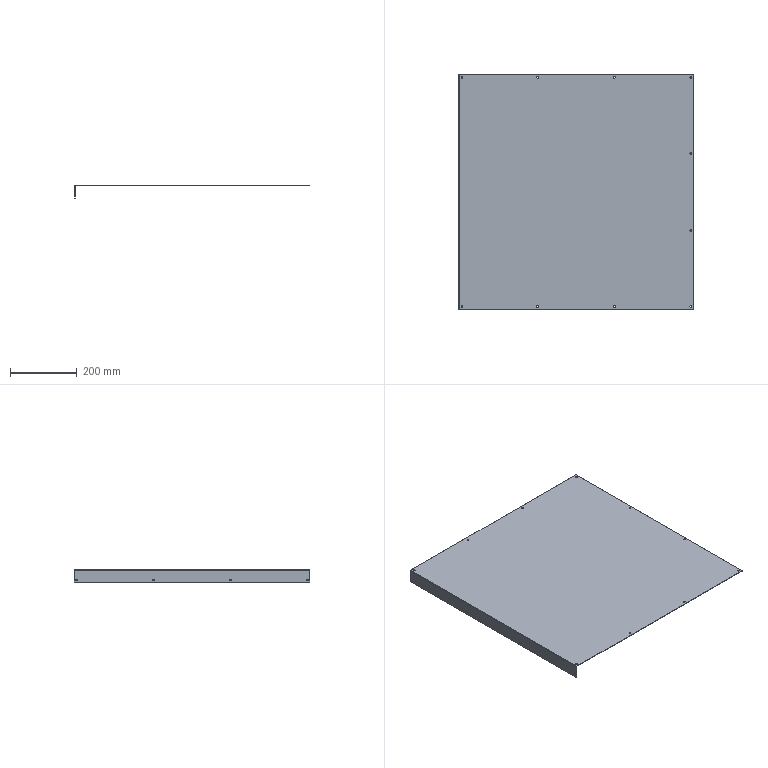Part | SolidWorks | features HoleWzd 2, EdgeFlange 1, Fillet 1, FlatPattern 1, SMBaseFlange 1, SheetMetal 1 | 1 solid | 46 faces | box 703 x 704 x 40 mm | volume 781813 mm3 | cylinder 34 | plane 12 | commonest cylinder face diameters 5 x29 4 x4 2 x1
STEP:
#1=CARTESIAN_POINT('',(-344.,-343.,-1.5));
#2=VERTEX_POINT('',#1);
#3=CARTESIAN_POINT('',(-339.,-343.,-1.5));
#4=VERTEX_POINT('',#3);
#5=CARTESIAN_POINT('',(-341.5,-343.,-1.5));
#6=DIRECTION('',(0.,0.,1.));
#7=DIRECTION('',(1.,0.,0.));
#8=AXIS2_PLACEMENT_3D('',#5,#6,#7);
#9=CIRCLE('',#8,2.5);
#10=EDGE_CURVE('',#2,#4,#9,.T.);
#11=ORIENTED_EDGE('',*,*,#10,.F.);
#12=CARTESIAN_POINT('',(-344.,-343.,0.));
#13=VERTEX_POINT('',#12);
#14=CARTESIAN_POINT('',(-344.,-343.,0.));
#15=DIRECTION('',(0.,0.,1.));
#16=VECTOR('',#15,1000.);
#17=LINE('',#14,#16);
#18=EDGE_CURVE('',#2,#13,#17,.T.);
#19=ORIENTED_EDGE('',*,*,#18,.T.);
#20=CARTESIAN_POINT('',(-339.,-343.,0.));
#21=VERTEX_POINT('',#20);
#22=CARTESIAN_POINT('',(-341.5,-343.,0.));
#23=DIRECTION('',(0.,0.,1.));
#24=DIRECTION('',(1.,0.,0.));
#25=AXIS2_PLACEMENT_3D('',#22,#23,#24);
#26=CIRCLE('',#25,2.5);
#27=EDGE_CURVE('',#13,#21,#26,.T.);
#28=ORIENTED_EDGE('',*,*,#27,.T.);
#29=CARTESIAN_POINT('',(-339.,-343.,0.));
#30=DIRECTION('',(0.,0.,1.));
#31=VECTOR('',#30,1000.);
#32=LINE('',#29,#31);
#33=EDGE_CURVE('',#4,#21,#32,.T.);
#34=ORIENTED_EDGE('',*,*,#33,.F.);
#35=EDGE_LOOP('',(#11,#19,#28,#34));
#36=FACE_OUTER_BOUND('',#35,.T.);
#37=CARTESIAN_POINT('',(-341.5,-343.,0.));
#38=DIRECTION('',(0.,0.,1.));
#39=DIRECTION('',(1.,0.,0.));
#40=AXIS2_PLACEMENT_3D('',#37,#38,#39);
#41=CYLINDRICAL_SURFACE('',#40,2.5);
#42=ADVANCED_FACE('',(#36),#41,.F.);
#43=CARTESIAN_POINT('',(-117.5,-343.,-1.5));
#44=VERTEX_POINT('',#43);
#45=CARTESIAN_POINT('',(-112.5,-343.,-1.5));
#46=VERTEX_POINT('',#45);
#47=CARTESIAN_POINT('',(-115.,-343.,-1.5));
#48=DIRECTION('',(0.,0.,1.));
#49=DIRECTION('',(1.,0.,0.));
#50=AXIS2_PLACEMENT_3D('',#47,#48,#49);
#51=CIRCLE('',#50,2.5);
#52=EDGE_CURVE('',#44,#46,#51,.T.);
#53=ORIENTED_EDGE('',*,*,#52,.F.);
#54=CARTESIAN_POINT('',(-117.5,-343.,0.));
#55=VERTEX_POINT('',#54);
#56=CARTESIAN_POINT('',(-117.5,-343.,0.));
#57=DIRECTION('',(0.,0.,1.));
#58=VECTOR('',#57,1000.);
#59=LINE('',#56,#58);
#60=EDGE_CURVE('',#44,#55,#59,.T.);
#61=ORIENTED_EDGE('',*,*,#60,.T.);
#62=CARTESIAN_POINT('',(-112.5,-343.,0.));
#63=VERTEX_POINT('',#62);
#64=CARTESIAN_POINT('',(-115.,-343.,0.));
#65=DIRECTION('',(0.,0.,1.));
#66=DIRECTION('',(1.,0.,0.));
#67=AXIS2_PLACEMENT_3D('',#64,#65,#66);
#68=CIRCLE('',#67,2.5);
#69=EDGE_CURVE('',#55,#63,#68,.T.);
#70=ORIENTED_EDGE('',*,*,#69,.T.);
#71=CARTESIAN_POINT('',(-112.5,-343.,0.));
#72=DIRECTION('',(0.,0.,1.));
#73=VECTOR('',#72,1000.);
#74=LINE('',#71,#73);
#75=EDGE_CURVE('',#46,#63,#74,.T.);
#76=ORIENTED_EDGE('',*,*,#75,.F.);
#77=EDGE_LOOP('',(#53,#61,#70,#76));
#78=FACE_OUTER_BOUND('',#77,.T.);
#79=CARTESIAN_POINT('',(-115.,-343.,0.));
#80=DIRECTION('',(0.,0.,1.));
#81=DIRECTION('',(1.,0.,0.));
#82=AXIS2_PLACEMENT_3D('',#79,#80,#81);
#83=CYLINDRICAL_SURFACE('',#82,2.5);
#84=ADVANCED_FACE('',(#78),#83,.F.);
#85=CARTESIAN_POINT('',(112.5,-343.,-1.5));
#86=VERTEX_POINT('',#85);
#87=CARTESIAN_POINT('',(117.5,-343.,-1.5));
#88=VERTEX_POINT('',#87);
#89=CARTESIAN_POINT('',(115.,-343.,-1.5));
#90=DIRECTION('',(0.,0.,1.));
#91=DIRECTION('',(1.,0.,0.));
#92=AXIS2_PLACEMENT_3D('',#89,#90,#91);
#93=CIRCLE('',#92,2.5);
#94=EDGE_CURVE('',#86,#88,#93,.T.);
#95=ORIENTED_EDGE('',*,*,#94,.F.);
#96=CARTESIAN_POINT('',(112.5,-343.,0.));
#97=VERTEX_POINT('',#96);
#98=CARTESIAN_POINT('',(112.5,-343.,0.));
#99=DIRECTION('',(0.,0.,1.));
#100=VECTOR('',#99,1000.);
#101=LINE('',#98,#100);
#102=EDGE_CURVE('',#86,#97,#101,.T.);
#103=ORIENTED_EDGE('',*,*,#102,.T.);
#104=CARTESIAN_POINT('',(117.5,-343.,0.));
#105=VERTEX_POINT('',#104);
#106=CARTESIAN_POINT('',(115.,-343.,0.));
#107=DIRECTION('',(0.,0.,1.));
#108=DIRECTION('',(1.,0.,0.));
#109=AXIS2_PLACEMENT_3D('',#106,#107,#108);
#110=CIRCLE('',#109,2.5);
#111=EDGE_CURVE('',#97,#105,#110,.T.);
#112=ORIENTED_EDGE('',*,*,#111,.T.);
#113=CARTESIAN_POINT('',(117.5,-343.,0.));
#114=DIRECTION('',(0.,0.,1.));
#115=VECTOR('',#114,1000.);
#116=LINE('',#113,#115);
#117=EDGE_CURVE('',#88,#105,#116,.T.);
#118=ORIENTED_EDGE('',*,*,#117,.F.);
#119=EDGE_LOOP('',(#95,#103,#112,#118));
#120=FACE_OUTER_BOUND('',#119,.T.);
#121=CARTESIAN_POINT('',(115.,-343.,0.));
#122=DIRECTION('',(0.,0.,1.));
#123=DIRECTION('',(1.,0.,0.));
#124=AXIS2_PLACEMENT_3D('',#121,#122,#123);
#125=CYLINDRICAL_SURFACE('',#124,2.5);
#126=ADVANCED_FACE('',(#120),#125,.F.);
#127=CARTESIAN_POINT('',(341.,-343.,-1.5));
#128=VERTEX_POINT('',#127);
#129=CARTESIAN_POINT('',(346.,-343.,-1.5));
#130=VERTEX_POINT('',#129);
#131=CARTESIAN_POINT('',(343.5,-343.,-1.5));
#132=DIRECTION('',(0.,0.,1.));
#133=DIRECTION('',(1.,0.,0.));
#134=AXIS2_PLACEMENT_3D('',#131,#132,#133);
#135=CIRCLE('',#134,2.5);
#136=EDGE_CURVE('',#128,#130,#135,.T.);
#137=ORIENTED_EDGE('',*,*,#136,.F.);
#138=CARTESIAN_POINT('',(341.,-343.,0.));
#139=VERTEX_POINT('',#138);
#140=CARTESIAN_POINT('',(341.,-343.,0.));
#141=DIRECTION('',(0.,0.,1.));
#142=VECTOR('',#141,1000.);
#143=LINE('',#140,#142);
#144=EDGE_CURVE('',#128,#139,#143,.T.);
#145=ORIENTED_EDGE('',*,*,#144,.T.);
#146=CARTESIAN_POINT('',(346.,-343.,0.));
#147=VERTEX_POINT('',#146);
#148=CARTESIAN_POINT('',(343.5,-343.,0.));
#149=DIRECTION('',(0.,0.,1.));
#150=DIRECTION('',(1.,0.,0.));
#151=AXIS2_PLACEMENT_3D('',#148,#149,#150);
#152=CIRCLE('',#151,2.5);
#153=EDGE_CURVE('',#139,#147,#152,.T.);
#154=ORIENTED_EDGE('',*,*,#153,.T.);
#155=CARTESIAN_POINT('',(346.,-343.,0.));
#156=DIRECTION('',(0.,0.,1.));
#157=VECTOR('',#156,1000.);
#158=LINE('',#155,#157);
#159=EDGE_CURVE('',#130,#147,#158,.T.);
#160=ORIENTED_EDGE('',*,*,#159,.F.);
#161=EDGE_LOOP('',(#137,#145,#154,#160));
#162=FACE_OUTER_BOUND('',#161,.T.);
#163=CARTESIAN_POINT('',(343.5,-343.,0.));
#164=DIRECTION('',(0.,0.,1.));
#165=DIRECTION('',(1.,0.,0.));
#166=AXIS2_PLACEMENT_3D('',#163,#164,#165);
#167=CYLINDRICAL_SURFACE('',#166,2.5);
#168=ADVANCED_FACE('',(#162),#167,.F.);
#169=CARTESIAN_POINT('',(341.,-115.,-1.5));
#170=VERTEX_POINT('',#169);
#171=CARTESIAN_POINT('',(346.,-115.,-1.5));
#172=VERTEX_POINT('',#171);
#173=CARTESIAN_POINT('',(343.5,-115.,-1.5));
#174=DIRECTION('',(0.,0.,1.));
#175=DIRECTION('',(1.,0.,0.));
#176=AXIS2_PLACEMENT_3D('',#173,#174,#175);
#177=CIRCLE('',#176,2.5);
#178=EDGE_CURVE('',#170,#172,#177,.T.);
#179=ORIENTED_EDGE('',*,*,#178,.F.);
#180=CARTESIAN_POINT('',(341.,-115.,0.));
#181=VERTEX_POINT('',#180);
#182=CARTESIAN_POINT('',(341.,-115.,0.));
#183=DIRECTION('',(0.,0.,1.));
#184=VECTOR('',#183,1000.);
#185=LINE('',#182,#184);
#186=EDGE_CURVE('',#170,#181,#185,.T.);
#187=ORIENTED_EDGE('',*,*,#186,.T.);
#188=CARTESIAN_POINT('',(346.,-115.,0.));
#189=VERTEX_POINT('',#188);
#190=CARTESIAN_POINT('',(343.5,-115.,0.));
#191=DIRECTION('',(0.,0.,1.));
#192=DIRECTION('',(1.,0.,0.));
#193=AXIS2_PLACEMENT_3D('',#190,#191,#192);
#194=CIRCLE('',#193,2.5);
#195=EDGE_CURVE('',#181,#189,#194,.T.);
#196=ORIENTED_EDGE('',*,*,#195,.T.);
#197=CARTESIAN_POINT('',(346.,-115.,0.));
#198=DIRECTION('',(0.,0.,1.));
#199=VECTOR('',#198,1000.);
#200=LINE('',#197,#199);
#201=EDGE_CURVE('',#172,#189,#200,.T.);
#202=ORIENTED_EDGE('',*,*,#201,.F.);
#203=EDGE_LOOP('',(#179,#187,#196,#202));
#204=FACE_OUTER_BOUND('',#203,.T.);
#205=CARTESIAN_POINT('',(343.5,-115.,0.));
#206=DIRECTION('',(0.,0.,1.));
#207=DIRECTION('',(1.,0.,0.));
#208=AXIS2_PLACEMENT_3D('',#205,#206,#207);
#209=CYLINDRICAL_SURFACE('',#208,2.5);
#210=ADVANCED_FACE('',(#204),#209,.F.);
#211=CARTESIAN_POINT('',(341.,115.,-1.5));
#212=VERTEX_POINT('',#211);
#213=CARTESIAN_POINT('',(346.,115.,-1.5));
#214=VERTEX_POINT('',#213);
#215=CARTESIAN_POINT('',(343.5,115.,-1.5));
#216=DIRECTION('',(0.,0.,1.));
#217=DIRECTION('',(1.,0.,0.));
#218=AXIS2_PLACEMENT_3D('',#215,#216,#217);
#219=CIRCLE('',#218,2.5);
#220=EDGE_CURVE('',#212,#214,#219,.T.);
#221=ORIENTED_EDGE('',*,*,#220,.F.);
#222=CARTESIAN_POINT('',(341.,115.,0.));
#223=VERTEX_POINT('',#222);
#224=CARTESIAN_POINT('',(341.,115.,0.));
#225=DIRECTION('',(0.,0.,1.));
#226=VECTOR('',#225,1000.);
#227=LINE('',#224,#226);
#228=EDGE_CURVE('',#212,#223,#227,.T.);
#229=ORIENTED_EDGE('',*,*,#228,.T.);
#230=CARTESIAN_POINT('',(346.,115.,0.));
#231=VERTEX_POINT('',#230);
#232=CARTESIAN_POINT('',(343.5,115.,0.));
#233=DIRECTION('',(0.,0.,1.));
#234=DIRECTION('',(1.,0.,0.));
#235=AXIS2_PLACEMENT_3D('',#232,#233,#234);
#236=CIRCLE('',#235,2.5);
#237=EDGE_CURVE('',#223,#231,#236,.T.);
#238=ORIENTED_EDGE('',*,*,#237,.T.);
#239=CARTESIAN_POINT('',(346.,115.,0.));
#240=DIRECTION('',(0.,0.,1.));
#241=VECTOR('',#240,1000.);
#242=LINE('',#239,#241);
#243=EDGE_CURVE('',#214,#231,#242,.T.);
#244=ORIENTED_EDGE('',*,*,#243,.F.);
#245=EDGE_LOOP('',(#221,#229,#238,#244));
#246=FACE_OUTER_BOUND('',#245,.T.);
#247=CARTESIAN_POINT('',(343.5,115.,0.));
#248=DIRECTION('',(0.,0.,1.));
#249=DIRECTION('',(1.,0.,0.));
#250=AXIS2_PLACEMENT_3D('',#247,#248,#249);
#251=CYLINDRICAL_SURFACE('',#250,2.5);
#252=ADVANCED_FACE('',(#246),#251,.F.);
#253=CARTESIAN_POINT('',(341.,343.,-1.5));
#254=VERTEX_POINT('',#253);
#255=CARTESIAN_POINT('',(346.,343.,-1.5));
#256=VERTEX_POINT('',#255);
#257=CARTESIAN_POINT('',(343.5,343.,-1.5));
#258=DIRECTION('',(0.,0.,1.));
#259=DIRECTION('',(1.,0.,0.));
#260=AXIS2_PLACEMENT_3D('',#257,#258,#259);
#261=CIRCLE('',#260,2.5);
#262=EDGE_CURVE('',#254,#256,#261,.T.);
#263=ORIENTED_EDGE('',*,*,#262,.F.);
#264=CARTESIAN_POINT('',(341.,343.,0.));
#265=VERTEX_POINT('',#264);
#266=CARTESIAN_POINT('',(341.,343.,0.));
#267=DIRECTION('',(0.,0.,1.));
#268=VECTOR('',#267,1000.);
#269=LINE('',#266,#268);
#270=EDGE_CURVE('',#254,#265,#269,.T.);
#271=ORIENTED_EDGE('',*,*,#270,.T.);
#272=CARTESIAN_POINT('',(346.,343.,0.));
#273=VERTEX_POINT('',#272);
#274=CARTESIAN_POINT('',(343.5,343.,0.));
#275=DIRECTION('',(0.,0.,1.));
#276=DIRECTION('',(1.,0.,0.));
#277=AXIS2_PLACEMENT_3D('',#274,#275,#276);
#278=CIRCLE('',#277,2.5);
#279=EDGE_CURVE('',#265,#273,#278,.T.);
#280=ORIENTED_EDGE('',*,*,#279,.T.);
#281=CARTESIAN_POINT('',(346.,343.,0.));
#282=DIRECTION('',(0.,0.,1.));
#283=VECTOR('',#282,1000.);
#284=LINE('',#281,#283);
#285=EDGE_CURVE('',#256,#273,#284,.T.);
#286=ORIENTED_EDGE('',*,*,#285,.F.);
#287=EDGE_LOOP('',(#263,#271,#280,#286));
#288=FACE_OUTER_BOUND('',#287,.T.);
#289=CARTESIAN_POINT('',(343.5,343.,0.));
#290=DIRECTION('',(0.,0.,1.));
#291=DIRECTION('',(1.,0.,0.));
#292=AXIS2_PLACEMENT_3D('',#289,#290,#291);
#293=CYLINDRICAL_SURFACE('',#292,2.5);
#294=ADVANCED_FACE('',(#288),#293,.F.);
#295=CARTESIAN_POINT('',(112.5,343.,-1.5));
#296=VERTEX_POINT('',#295);
#297=CARTESIAN_POINT('',(117.5,343.,-1.5));
#298=VERTEX_POINT('',#297);
#299=CARTESIAN_POINT('',(115.,343.,-1.5));
#300=DIRECTION('',(0.,0.,1.));
#301=DIRECTION('',(1.,0.,0.));
#302=AXIS2_PLACEMENT_3D('',#299,#300,#301);
#303=CIRCLE('',#302,2.5);
#304=EDGE_CURVE('',#296,#298,#303,.T.);
#305=ORIENTED_EDGE('',*,*,#304,.F.);
#306=CARTESIAN_POINT('',(112.5,343.,0.));
#307=VERTEX_POINT('',#306);
#308=CARTESIAN_POINT('',(112.5,343.,0.));
#309=DIRECTION('',(0.,0.,1.));
#310=VECTOR('',#309,1000.);
#311=LINE('',#308,#310);
#312=EDGE_CURVE('',#296,#307,#311,.T.);
#313=ORIENTED_EDGE('',*,*,#312,.T.);
#314=CARTESIAN_POINT('',(117.5,343.,0.));
#315=VERTEX_POINT('',#314);
#316=CARTESIAN_POINT('',(115.,343.,0.));
#317=DIRECTION('',(0.,0.,1.));
#318=DIRECTION('',(1.,0.,0.));
#319=AXIS2_PLACEMENT_3D('',#316,#317,#318);
#320=CIRCLE('',#319,2.5);
#321=EDGE_CURVE('',#307,#315,#320,.T.);
#322=ORIENTED_EDGE('',*,*,#321,.T.);
#323=CARTESIAN_POINT('',(117.5,343.,0.));
#324=DIRECTION('',(0.,0.,1.));
#325=VECTOR('',#324,1000.);
#326=LINE('',#323,#325);
#327=EDGE_CURVE('',#298,#315,#326,.T.);
#328=ORIENTED_EDGE('',*,*,#327,.F.);
#329=EDGE_LOOP('',(#305,#313,#322,#328));
#330=FACE_OUTER_BOUND('',#329,.T.);
#331=CARTESIAN_POINT('',(115.,343.,0.));
#332=DIRECTION('',(0.,0.,1.));
#333=DIRECTION('',(1.,0.,0.));
#334=AXIS2_PLACEMENT_3D('',#331,#332,#333);
#335=CYLINDRICAL_SURFACE('',#334,2.5);
#336=ADVANCED_FACE('',(#330),#335,.F.);
#337=CARTESIAN_POINT('',(-117.5,343.,-1.5));
#338=VERTEX_POINT('',#337);
#339=CARTESIAN_POINT('',(-112.5,343.,-1.5));
#340=VERTEX_POINT('',#339);
#341=CARTESIAN_POINT('',(-115.,343.,-1.5));
#342=DIRECTION('',(0.,0.,1.));
#343=DIRECTION('',(1.,0.,0.));
#344=AXIS2_PLACEMENT_3D('',#341,#342,#343);
#345=CIRCLE('',#344,2.5);
#346=EDGE_CURVE('',#338,#340,#345,.T.);
#347=ORIENTED_EDGE('',*,*,#346,.F.);
#348=CARTESIAN_POINT('',(-117.5,343.,0.));
#349=VERTEX_POINT('',#348);
#350=CARTESIAN_POINT('',(-117.5,343.,0.));
#351=DIRECTION('',(0.,0.,1.));
#352=VECTOR('',#351,1000.);
#353=LINE('',#350,#352);
#354=EDGE_CURVE('',#338,#349,#353,.T.);
#355=ORIENTED_EDGE('',*,*,#354,.T.);
#356=CARTESIAN_POINT('',(-112.5,343.,0.));
#357=VERTEX_POINT('',#356);
#358=CARTESIAN_POINT('',(-115.,343.,0.));
#359=DIRECTION('',(0.,0.,1.));
#360=DIRECTION('',(1.,0.,0.));
#361=AXIS2_PLACEMENT_3D('',#358,#359,#360);
#362=CIRCLE('',#361,2.5);
#363=EDGE_CURVE('',#349,#357,#362,.T.);
#364=ORIENTED_EDGE('',*,*,#363,.T.);
#365=CARTESIAN_POINT('',(-112.5,343.,0.));
#366=DIRECTION('',(0.,0.,1.));
#367=VECTOR('',#366,1000.);
#368=LINE('',#365,#367);
#369=EDGE_CURVE('',#340,#357,#368,.T.);
#370=ORIENTED_EDGE('',*,*,#369,.F.);
#371=EDGE_LOOP('',(#347,#355,#364,#370));
#372=FACE_OUTER_BOUND('',#371,.T.);
#373=CARTESIAN_POINT('',(-115.,343.,0.));
#374=DIRECTION('',(0.,0.,1.));
#375=DIRECTION('',(1.,0.,0.));
#376=AXIS2_PLACEMENT_3D('',#373,#374,#375);
#377=CYLINDRICAL_SURFACE('',#376,2.5);
#378=ADVANCED_FACE('',(#372),#377,.F.);
#379=CARTESIAN_POINT('',(-344.,343.,-1.5));
#380=VERTEX_POINT('',#379);
#381=CARTESIAN_POINT('',(-339.,343.,-1.5));
#382=VERTEX_POINT('',#381);
#383=CARTESIAN_POINT('',(-341.5,343.,-1.5));
#384=DIRECTION('',(0.,0.,1.));
#385=DIRECTION('',(1.,0.,0.));
#386=AXIS2_PLACEMENT_3D('',#383,#384,#385);
#387=CIRCLE('',#386,2.5);
#388=EDGE_CURVE('',#380,#382,#387,.T.);
#389=ORIENTED_EDGE('',*,*,#388,.F.);
#390=CARTESIAN_POINT('',(-344.,343.,0.));
#391=VERTEX_POINT('',#390);
#392=CARTESIAN_POINT('',(-344.,343.,0.));
#393=DIRECTION('',(0.,0.,1.));
#394=VECTOR('',#393,1000.);
#395=LINE('',#392,#394);
#396=EDGE_CURVE('',#380,#391,#395,.T.);
#397=ORIENTED_EDGE('',*,*,#396,.T.);
#398=CARTESIAN_POINT('',(-339.,343.,0.));
#399=VERTEX_POINT('',#398);
#400=CARTESIAN_POINT('',(-341.5,343.,0.));
#401=DIRECTION('',(0.,0.,1.));
#402=DIRECTION('',(1.,0.,0.));
#403=AXIS2_PLACEMENT_3D('',#400,#401,#402);
#404=CIRCLE('',#403,2.5);
#405=EDGE_CURVE('',#391,#399,#404,.T.);
#406=ORIENTED_EDGE('',*,*,#405,.T.);
#407=CARTESIAN_POINT('',(-339.,343.,0.));
#408=DIRECTION('',(0.,0.,1.));
#409=VECTOR('',#408,1000.);
#410=LINE('',#407,#409);
#411=EDGE_CURVE('',#382,#399,#410,.T.);
#412=ORIENTED_EDGE('',*,*,#411,.F.);
#413=EDGE_LOOP('',(#389,#397,#406,#412));
#414=FACE_OUTER_BOUND('',#413,.T.);
#415=CARTESIAN_POINT('',(-341.5,343.,0.));
#416=DIRECTION('',(0.,0.,1.));
#417=DIRECTION('',(1.,0.,0.));
#418=AXIS2_PLACEMENT_3D('',#415,#416,#417);
#419=CYLINDRICAL_SURFACE('',#418,2.5);
#420=ADVANCED_FACE('',(#414),#419,.F.);
#421=CARTESIAN_POINT('',(-350.,346.,-34.5));
#422=VERTEX_POINT('',#421);
#423=CARTESIAN_POINT('',(-350.,346.,-29.5));
#424=VERTEX_POINT('',#423);
#425=CARTESIAN_POINT('',(-350.,346.,-32.));
#426=DIRECTION('',(-1.,0.,0.));
#427=DIRECTION('',(0.,0.,1.));
#428=AXIS2_PLACEMENT_3D('',#425,#426,#427);
#429=CIRCLE('',#428,2.5);
#430=EDGE_CURVE('',#422,#424,#429,.T.);
#431=ORIENTED_EDGE('',*,*,#430,.F.);
#432=CARTESIAN_POINT('',(-351.5,346.,-34.5));
#433=VERTEX_POINT('',#432);
#434=CARTESIAN_POINT('',(-351.5,346.,-34.5));
#435=DIRECTION('',(-1.,0.,0.));
#436=VECTOR('',#435,1000.);
#437=LINE('',#434,#436);
#438=EDGE_CURVE('',#422,#433,#437,.T.);
#439=ORIENTED_EDGE('',*,*,#438,.T.);
#440=CARTESIAN_POINT('',(-351.5,346.,-29.5));
#441=VERTEX_POINT('',#440);
#442=CARTESIAN_POINT('',(-351.5,346.,-32.));
#443=DIRECTION('',(-1.,0.,0.));
#444=DIRECTION('',(0.,0.,1.));
#445=AXIS2_PLACEMENT_3D('',#442,#443,#444);
#446=CIRCLE('',#445,2.5);
#447=EDGE_CURVE('',#433,#441,#446,.T.);
#448=ORIENTED_EDGE('',*,*,#447,.T.);
#449=CARTESIAN_POINT('',(-351.5,346.,-29.5));
#450=DIRECTION('',(-1.,0.,0.));
#451=VECTOR('',#450,1000.);
#452=LINE('',#449,#451);
#453=EDGE_CURVE('',#424,#441,#452,.T.);
#454=ORIENTED_EDGE('',*,*,#453,.F.);
#455=EDGE_LOOP('',(#431,#439,#448,#454));
#456=FACE_OUTER_BOUND('',#455,.T.);
#457=CARTESIAN_POINT('',(-351.5,346.,-32.));
#458=DIRECTION('',(-1.,0.,0.));
#459=DIRECTION('',(0.,0.,1.));
#460=AXIS2_PLACEMENT_3D('',#457,#458,#459);
#461=CYLINDRICAL_SURFACE('',#460,2.5);
#462=ADVANCED_FACE('',(#456),#461,.F.);
#463=CARTESIAN_POINT('',(-350.,115.,-34.5));
#464=VERTEX_POINT('',#463);
#465=CARTESIAN_POINT('',(-350.,115.,-29.5));
#466=VERTEX_POINT('',#465);
#467=CARTESIAN_POINT('',(-350.,115.,-32.));
#468=DIRECTION('',(-1.,0.,0.));
#469=DIRECTION('',(0.,0.,1.));
#470=AXIS2_PLACEMENT_3D('',#467,#468,#469);
#471=CIRCLE('',#470,2.5);
#472=EDGE_CURVE('',#464,#466,#471,.T.);
#473=ORIENTED_EDGE('',*,*,#472,.F.);
#474=CARTESIAN_POINT('',(-351.5,115.,-34.5));
#475=VERTEX_POINT('',#474);
#476=CARTESIAN_POINT('',(-351.5,115.,-34.5));
#477=DIRECTION('',(-1.,0.,0.));
#478=VECTOR('',#477,1000.);
#479=LINE('',#476,#478);
#480=EDGE_CURVE('',#464,#475,#479,.T.);
#481=ORIENTED_EDGE('',*,*,#480,.T.);
#482=CARTESIAN_POINT('',(-351.5,115.,-29.5));
#483=VERTEX_POINT('',#482);
#484=CARTESIAN_POINT('',(-351.5,115.,-32.));
#485=DIRECTION('',(-1.,0.,0.));
#486=DIRECTION('',(0.,0.,1.));
#487=AXIS2_PLACEMENT_3D('',#484,#485,#486);
#488=CIRCLE('',#487,2.5);
#489=EDGE_CURVE('',#475,#483,#488,.T.);
#490=ORIENTED_EDGE('',*,*,#489,.T.);
#491=CARTESIAN_POINT('',(-351.5,115.,-29.5));
#492=DIRECTION('',(-1.,0.,0.));
#493=VECTOR('',#492,1000.);
#494=LINE('',#491,#493);
#495=EDGE_CURVE('',#466,#483,#494,.T.);
#496=ORIENTED_EDGE('',*,*,#495,.F.);
#497=EDGE_LOOP('',(#473,#481,#490,#496));
#498=FACE_OUTER_BOUND('',#497,.T.);
#499=CARTESIAN_POINT('',(-351.5,115.,-32.));
#500=DIRECTION('',(-1.,0.,0.));
#501=DIRECTION('',(0.,0.,1.));
#502=AXIS2_PLACEMENT_3D('',#499,#500,#501);
#503=CYLINDRICAL_SURFACE('',#502,2.5);
#504=ADVANCED_FACE('',(#498),#503,.F.);
#505=CARTESIAN_POINT('',(-350.,-346.,-34.5));
#506=VERTEX_POINT('',#505);
#507=CARTESIAN_POINT('',(-350.,-346.,-29.5));
#508=VERTEX_POINT('',#507);
#509=CARTESIAN_POINT('',(-350.,-346.,-32.));
#510=DIRECTION('',(-1.,0.,0.));
#511=DIRECTION('',(0.,0.,1.));
#512=AXIS2_PLACEMENT_3D('',#509,#510,#511);
#513=CIRCLE('',#512,2.5);
#514=EDGE_CURVE('',#506,#508,#513,.T.);
#515=ORIENTED_EDGE('',*,*,#514,.F.);
#516=CARTESIAN_POINT('',(-351.5,-346.,-34.5));
#517=VERTEX_POINT('',#516);
#518=CARTESIAN_POINT('',(-351.5,-346.,-34.5));
#519=DIRECTION('',(-1.,0.,0.));
#520=VECTOR('',#519,1000.);
#521=LINE('',#518,#520);
#522=EDGE_CURVE('',#506,#517,#521,.T.);
#523=ORIENTED_EDGE('',*,*,#522,.T.);
#524=CARTESIAN_POINT('',(-351.5,-346.,-29.5));
#525=VERTEX_POINT('',#524);
#526=CARTESIAN_POINT('',(-351.5,-346.,-32.));
#527=DIRECTION('',(-1.,0.,0.));
#528=DIRECTION('',(0.,0.,1.));
#529=AXIS2_PLACEMENT_3D('',#526,#527,#528);
#530=CIRCLE('',#529,2.5);
#531=EDGE_CURVE('',#517,#525,#530,.T.);
#532=ORIENTED_EDGE('',*,*,#531,.T.);
#533=CARTESIAN_POINT('',(-351.5,-346.,-29.5));
#534=DIRECTION('',(-1.,0.,0.));
#535=VECTOR('',#534,1000.);
#536=LINE('',#533,#535);
#537=EDGE_CURVE('',#508,#525,#536,.T.);
#538=ORIENTED_EDGE('',*,*,#537,.F.);
#539=EDGE_LOOP('',(#515,#523,#532,#538));
#540=FACE_OUTER_BOUND('',#539,.T.);
#541=CARTESIAN_POINT('',(-351.5,-346.,-32.));
#542=DIRECTION('',(-1.,0.,0.));
#543=DIRECTION('',(0.,0.,1.));
#544=AXIS2_PLACEMENT_3D('',#541,#542,#543);
#545=CYLINDRICAL_SURFACE('',#544,2.5);
#546=ADVANCED_FACE('',(#540),#545,.F.);
#547=CARTESIAN_POINT('',(-350.,-115.,-34.5));
#548=VERTEX_POINT('',#547);
#549=CARTESIAN_POINT('',(-350.,-115.,-29.5));
#550=VERTEX_POINT('',#549);
#551=CARTESIAN_POINT('',(-350.,-115.,-32.));
#552=DIRECTION('',(-1.,0.,0.));
#553=DIRECTION('',(0.,0.,1.));
#554=AXIS2_PLACEMENT_3D('',#551,#552,#553);
#555=CIRCLE('',#554,2.5);
#556=EDGE_CURVE('',#548,#550,#555,.T.);
#557=ORIENTED_EDGE('',*,*,#556,.F.);
#558=CARTESIAN_POINT('',(-351.5,-115.,-34.5));
#559=VERTEX_POINT('',#558);
#560=CARTESIAN_POINT('',(-351.5,-115.,-34.5));
#561=DIRECTION('',(-1.,0.,0.));
#562=VECTOR('',#561,1000.);
#563=LINE('',#560,#562);
#564=EDGE_CURVE('',#548,#559,#563,.T.);
#565=ORIENTED_EDGE('',*,*,#564,.T.);
#566=CARTESIAN_POINT('',(-351.5,-115.,-29.5));
#567=VERTEX_POINT('',#566);
#568=CARTESIAN_POINT('',(-351.5,-115.,-32.));
#569=DIRECTION('',(-1.,0.,0.));
#570=DIRECTION('',(0.,0.,1.));
#571=AXIS2_PLACEMENT_3D('',#568,#569,#570);
#572=CIRCLE('',#571,2.5);
#573=EDGE_CURVE('',#559,#567,#572,.T.);
#574=ORIENTED_EDGE('',*,*,#573,.T.);
#575=CARTESIAN_POINT('',(-351.5,-115.,-29.5));
#576=DIRECTION('',(-1.,0.,0.));
#577=VECTOR('',#576,1000.);
#578=LINE('',#575,#577);
#579=EDGE_CURVE('',#550,#567,#578,.T.);
#580=ORIENTED_EDGE('',*,*,#579,.F.);
#581=EDGE_LOOP('',(#557,#565,#574,#580));
#582=FACE_OUTER_BOUND('',#581,.T.);
#583=CARTESIAN_POINT('',(-351.5,-115.,-32.));
#584=DIRECTION('',(-1.,0.,0.));
#585=DIRECTION('',(0.,0.,1.));
#586=AXIS2_PLACEMENT_3D('',#583,#584,#585);
#587=CYLINDRICAL_SURFACE('',#586,2.5);
#588=ADVANCED_FACE('',(#582),#587,.F.);
#589=CARTESIAN_POINT('',(349.5,352.,0.));
#590=VERTEX_POINT('',#589);
#591=CARTESIAN_POINT('',(-349.,352.,0.));
#592=VERTEX_POINT('',#591);
#593=CARTESIAN_POINT('',(351.5,352.,0.));
#594=DIRECTION('',(-1.,0.,0.));
#595=VECTOR('',#594,1000.);
#596=LINE('',#593,#595);
#597=EDGE_CURVE('',#590,#592,#596,.T.);
#598=ORIENTED_EDGE('',*,*,#597,.F.);
#599=CARTESIAN_POINT('',(349.5,352.,-1.5));
#600=VERTEX_POINT('',#599);
#601=CARTESIAN_POINT('',(349.5,352.,-1.5));
#602=DIRECTION('',(0.,0.,-1.));
#603=VECTOR('',#602,1000.);
#604=LINE('',#601,#603);
#605=EDGE_CURVE('',#590,#600,#604,.T.);
#606=ORIENTED_EDGE('',*,*,#605,.T.);
#607=CARTESIAN_POINT('',(-349.,352.,-1.5));
#608=VERTEX_POINT('',#607);
#609=CARTESIAN_POINT('',(351.5,352.,-1.5));
#610=DIRECTION('',(-1.,0.,0.));
#611=VECTOR('',#610,1000.);
#612=LINE('',#609,#611);
#613=EDGE_CURVE('',#600,#608,#612,.T.);
#614=ORIENTED_EDGE('',*,*,#613,.T.);
#615=CARTESIAN_POINT('',(-349.,352.,-1.5));
#616=DIRECTION('',(0.,0.,1.));
#617=VECTOR('',#616,1000.);
#618=LINE('',#615,#617);
#619=EDGE_CURVE('',#608,#592,#618,.T.);
#620=ORIENTED_EDGE('',*,*,#619,.T.);
#621=EDGE_LOOP('',(#598,#606,#614,#620));
#622=FACE_OUTER_BOUND('',#621,.T.);
#623=CARTESIAN_POINT('',(351.5,352.,-1.5));
#624=DIRECTION('',(0.,1.,0.));
#625=DIRECTION('',(-1.,0.,0.));
#626=AXIS2_PLACEMENT_3D('',#623,#624,#625);
#627=PLANE('',#626);
#628=ADVANCED_FACE('',(#622),#627,.T.);
#629=CARTESIAN_POINT('',(-341.5,-343.,-1.5));
#630=DIRECTION('',(0.,0.,1.));
#631=DIRECTION('',(1.,0.,0.));
#632=AXIS2_PLACEMENT_3D('',#629,#630,#631);
#633=CIRCLE('',#632,2.5);
#634=EDGE_CURVE('',#4,#2,#633,.T.);
#635=ORIENTED_EDGE('',*,*,#634,.T.);
#636=ORIENTED_EDGE('',*,*,#10,.T.);
#637=EDGE_LOOP('',(#635,#636));
#638=FACE_BOUND('',#637,.T.);
#639=CARTESIAN_POINT('',(-115.,-343.,-1.5));
#640=DIRECTION('',(0.,0.,1.));
#641=DIRECTION('',(1.,0.,0.));
#642=AXIS2_PLACEMENT_3D('',#639,#640,#641);
#643=CIRCLE('',#642,2.5);
#644=EDGE_CURVE('',#46,#44,#643,.T.);
#645=ORIENTED_EDGE('',*,*,#644,.T.);
#646=ORIENTED_EDGE('',*,*,#52,.T.);
#647=EDGE_LOOP('',(#645,#646));
#648=FACE_BOUND('',#647,.T.);
#649=CARTESIAN_POINT('',(115.,-343.,-1.5));
#650=DIRECTION('',(0.,0.,1.));
#651=DIRECTION('',(1.,0.,0.));
#652=AXIS2_PLACEMENT_3D('',#649,#650,#651);
#653=CIRCLE('',#652,2.5);
#654=EDGE_CURVE('',#88,#86,#653,.T.);
#655=ORIENTED_EDGE('',*,*,#654,.T.);
#656=ORIENTED_EDGE('',*,*,#94,.T.);
#657=EDGE_LOOP('',(#655,#656));
#658=FACE_BOUND('',#657,.T.);
#659=CARTESIAN_POINT('',(343.5,-343.,-1.5));
#660=DIRECTION('',(0.,0.,1.));
#661=DIRECTION('',(1.,0.,0.));
#662=AXIS2_PLACEMENT_3D('',#659,#660,#661);
#663=CIRCLE('',#662,2.5);
#664=EDGE_CURVE('',#130,#128,#663,.T.);
#665=ORIENTED_EDGE('',*,*,#664,.T.);
#666=ORIENTED_EDGE('',*,*,#136,.T.);
#667=EDGE_LOOP('',(#665,#666));
#668=FACE_BOUND('',#667,.T.);
#669=CARTESIAN_POINT('',(343.5,-115.,-1.5));
#670=DIRECTION('',(0.,0.,1.));
#671=DIRECTION('',(1.,0.,0.));
#672=AXIS2_PLACEMENT_3D('',#669,#670,#671);
#673=CIRCLE('',#672,2.5);
#674=EDGE_CURVE('',#172,#170,#673,.T.);
#675=ORIENTED_EDGE('',*,*,#674,.T.);
#676=ORIENTED_EDGE('',*,*,#178,.T.);
#677=EDGE_LOOP('',(#675,#676));
#678=FACE_BOUND('',#677,.T.);
#679=CARTESIAN_POINT('',(343.5,115.,-1.5));
#680=DIRECTION('',(0.,0.,1.));
#681=DIRECTION('',(1.,0.,0.));
#682=AXIS2_PLACEMENT_3D('',#679,#680,#681);
#683=CIRCLE('',#682,2.5);
#684=EDGE_CURVE('',#214,#212,#683,.T.);
#685=ORIENTED_EDGE('',*,*,#684,.T.);
#686=ORIENTED_EDGE('',*,*,#220,.T.);
#687=EDGE_LOOP('',(#685,#686));
#688=FACE_BOUND('',#687,.T.);
#689=CARTESIAN_POINT('',(343.5,343.,-1.5));
#690=DIRECTION('',(0.,0.,1.));
#691=DIRECTION('',(1.,0.,0.));
#692=AXIS2_PLACEMENT_3D('',#689,#690,#691);
#693=CIRCLE('',#692,2.5);
#694=EDGE_CURVE('',#256,#254,#693,.T.);
#695=ORIENTED_EDGE('',*,*,#694,.T.);
#696=ORIENTED_EDGE('',*,*,#262,.T.);
#697=EDGE_LOOP('',(#695,#696));
#698=FACE_BOUND('',#697,.T.);
#699=CARTESIAN_POINT('',(115.,343.,-1.5));
#700=DIRECTION('',(0.,0.,1.));
#701=DIRECTION('',(1.,0.,0.));
#702=AXIS2_PLACEMENT_3D('',#699,#700,#701);
#703=CIRCLE('',#702,2.5);
#704=EDGE_CURVE('',#298,#296,#703,.T.);
#705=ORIENTED_EDGE('',*,*,#704,.T.);
#706=ORIENTED_EDGE('',*,*,#304,.T.);
#707=EDGE_LOOP('',(#705,#706));
#708=FACE_BOUND('',#707,.T.);
#709=CARTESIAN_POINT('',(-115.,343.,-1.5));
#710=DIRECTION('',(0.,0.,1.));
#711=DIRECTION('',(1.,0.,0.));
#712=AXIS2_PLACEMENT_3D('',#709,#710,#711);
#713=CIRCLE('',#712,2.5);
#714=EDGE_CURVE('',#340,#338,#713,.T.);
#715=ORIENTED_EDGE('',*,*,#714,.T.);
#716=ORIENTED_EDGE('',*,*,#346,.T.);
#717=EDGE_LOOP('',(#715,#716));
#718=FACE_BOUND('',#717,.T.);
#719=CARTESIAN_POINT('',(-341.5,343.,-1.5));
#720=DIRECTION('',(0.,0.,1.));
#721=DIRECTION('',(1.,0.,0.));
#722=AXIS2_PLACEMENT_3D('',#719,#720,#721);
#723=CIRCLE('',#722,2.5);
#724=EDGE_CURVE('',#382,#380,#723,.T.);
#725=ORIENTED_EDGE('',*,*,#724,.T.);
#726=ORIENTED_EDGE('',*,*,#388,.T.);
#727=EDGE_LOOP('',(#725,#726));
#728=FACE_BOUND('',#727,.T.);
#729=CARTESIAN_POINT('',(351.5,-350.,-1.5));
#730=VERTEX_POINT('',#729);
#731=CARTESIAN_POINT('',(351.5,350.,-1.5));
#732=VERTEX_POINT('',#731);
#733=CARTESIAN_POINT('',(351.5,-352.,-1.5));
#734=DIRECTION('',(0.,1.,0.));
#735=VECTOR('',#734,1000.);
#736=LINE('',#733,#735);
#737=EDGE_CURVE('',#730,#732,#736,.T.);
#738=ORIENTED_EDGE('',*,*,#737,.F.);
#739=CARTESIAN_POINT('',(349.5,-352.,-1.5));
#740=VERTEX_POINT('',#739);
#741=CARTESIAN_POINT('',(349.5,-350.,-1.5));
#742=DIRECTION('',(0.,0.,-1.));
#743=DIRECTION('',(1.,0.,0.));
#744=AXIS2_PLACEMENT_3D('',#741,#742,#743);
#745=CIRCLE('',#744,2.);
#746=EDGE_CURVE('',#730,#740,#745,.T.);
#747=ORIENTED_EDGE('',*,*,#746,.T.);
#748=CARTESIAN_POINT('',(-349.,-352.,-1.5));
#749=VERTEX_POINT('',#748);
#750=CARTESIAN_POINT('',(351.5,-352.,-1.5));
#751=DIRECTION('',(1.,0.,0.));
#752=VECTOR('',#751,1000.);
#753=LINE('',#750,#752);
#754=EDGE_CURVE('',#749,#740,#753,.T.);
#755=ORIENTED_EDGE('',*,*,#754,.F.);
#756=CARTESIAN_POINT('',(-349.,352.,-1.5));
#757=DIRECTION('',(0.,-1.,0.));
#758=VECTOR('',#757,1000.);
#759=LINE('',#756,#758);
#760=EDGE_CURVE('',#608,#749,#759,.T.);
#761=ORIENTED_EDGE('',*,*,#760,.F.);
#762=ORIENTED_EDGE('',*,*,#613,.F.);
#763=CARTESIAN_POINT('',(349.5,350.,-1.5));
#764=DIRECTION('',(0.,0.,-1.));
#765=DIRECTION('',(1.,0.,0.));
#766=AXIS2_PLACEMENT_3D('',#763,#764,#765);
#767=CIRCLE('',#766,2.);
#768=EDGE_CURVE('',#600,#732,#767,.T.);
#769=ORIENTED_EDGE('',*,*,#768,.T.);
#770=EDGE_LOOP('',(#738,#747,#755,#761,#762,#769));
#771=FACE_OUTER_BOUND('',#770,.T.);
#772=CARTESIAN_POINT('',(0.,0.,-1.5));
#773=DIRECTION('',(0.,0.,1.));
#774=DIRECTION('',(1.,0.,0.));
#775=AXIS2_PLACEMENT_3D('',#772,#773,#774);
#776=PLANE('',#775);
#777=ADVANCED_FACE('',(#638,#648,#658,#668,#678,#688,#698,#708,#718,#728,#771),#776,.F.);
#778=CARTESIAN_POINT('',(-341.5,-343.,0.));
#779=DIRECTION('',(0.,0.,1.));
#780=DIRECTION('',(1.,0.,0.));
#781=AXIS2_PLACEMENT_3D('',#778,#779,#780);
#782=CIRCLE('',#781,2.5);
#783=EDGE_CURVE('',#21,#13,#782,.T.);
#784=ORIENTED_EDGE('',*,*,#783,.F.);
#785=ORIENTED_EDGE('',*,*,#27,.F.);
#786=EDGE_LOOP('',(#784,#785));
#787=FACE_BOUND('',#786,.T.);
#788=CARTESIAN_POINT('',(-115.,-343.,0.));
#789=DIRECTION('',(0.,0.,1.));
#790=DIRECTION('',(1.,0.,0.));
#791=AXIS2_PLACEMENT_3D('',#788,#789,#790);
#792=CIRCLE('',#791,2.5);
#793=EDGE_CURVE('',#63,#55,#792,.T.);
#794=ORIENTED_EDGE('',*,*,#793,.F.);
#795=ORIENTED_EDGE('',*,*,#69,.F.);
#796=EDGE_LOOP('',(#794,#795));
#797=FACE_BOUND('',#796,.T.);
#798=CARTESIAN_POINT('',(115.,-343.,0.));
#799=DIRECTION('',(0.,0.,1.));
#800=DIRECTION('',(1.,0.,0.));
#801=AXIS2_PLACEMENT_3D('',#798,#799,#800);
#802=CIRCLE('',#801,2.5);
#803=EDGE_CURVE('',#105,#97,#802,.T.);
#804=ORIENTED_EDGE('',*,*,#803,.F.);
#805=ORIENTED_EDGE('',*,*,#111,.F.);
#806=EDGE_LOOP('',(#804,#805));
#807=FACE_BOUND('',#806,.T.);
#808=CARTESIAN_POINT('',(343.5,-343.,0.));
#809=DIRECTION('',(0.,0.,1.));
#810=DIRECTION('',(1.,0.,0.));
#811=AXIS2_PLACEMENT_3D('',#808,#809,#810);
#812=CIRCLE('',#811,2.5);
#813=EDGE_CURVE('',#147,#139,#812,.T.);
#814=ORIENTED_EDGE('',*,*,#813,.F.);
#815=ORIENTED_EDGE('',*,*,#153,.F.);
#816=EDGE_LOOP('',(#814,#815));
#817=FACE_BOUND('',#816,.T.);
#818=CARTESIAN_POINT('',(343.5,-115.,0.));
#819=DIRECTION('',(0.,0.,1.));
#820=DIRECTION('',(1.,0.,0.));
#821=AXIS2_PLACEMENT_3D('',#818,#819,#820);
#822=CIRCLE('',#821,2.5);
#823=EDGE_CURVE('',#189,#181,#822,.T.);
#824=ORIENTED_EDGE('',*,*,#823,.F.);
#825=ORIENTED_EDGE('',*,*,#195,.F.);
#826=EDGE_LOOP('',(#824,#825));
#827=FACE_BOUND('',#826,.T.);
#828=CARTESIAN_POINT('',(343.5,115.,0.));
#829=DIRECTION('',(0.,0.,1.));
#830=DIRECTION('',(1.,0.,0.));
#831=AXIS2_PLACEMENT_3D('',#828,#829,#830);
#832=CIRCLE('',#831,2.5);
#833=EDGE_CURVE('',#231,#223,#832,.T.);
#834=ORIENTED_EDGE('',*,*,#833,.F.);
#835=ORIENTED_EDGE('',*,*,#237,.F.);
#836=EDGE_LOOP('',(#834,#835));
#837=FACE_BOUND('',#836,.T.);
#838=CARTESIAN_POINT('',(343.5,343.,0.));
#839=DIRECTION('',(0.,0.,1.));
#840=DIRECTION('',(1.,0.,0.));
#841=AXIS2_PLACEMENT_3D('',#838,#839,#840);
#842=CIRCLE('',#841,2.5);
#843=EDGE_CURVE('',#273,#265,#842,.T.);
#844=ORIENTED_EDGE('',*,*,#843,.F.);
#845=ORIENTED_EDGE('',*,*,#279,.F.);
#846=EDGE_LOOP('',(#844,#845));
#847=FACE_BOUND('',#846,.T.);
#848=CARTESIAN_POINT('',(115.,343.,0.));
#849=DIRECTION('',(0.,0.,1.));
#850=DIRECTION('',(1.,0.,0.));
#851=AXIS2_PLACEMENT_3D('',#848,#849,#850);
#852=CIRCLE('',#851,2.5);
#853=EDGE_CURVE('',#315,#307,#852,.T.);
#854=ORIENTED_EDGE('',*,*,#853,.F.);
#855=ORIENTED_EDGE('',*,*,#321,.F.);
#856=EDGE_LOOP('',(#854,#855));
#857=FACE_BOUND('',#856,.T.);
#858=CARTESIAN_POINT('',(-115.,343.,0.));
#859=DIRECTION('',(0.,0.,1.));
#860=DIRECTION('',(1.,0.,0.));
#861=AXIS2_PLACEMENT_3D('',#858,#859,#860);
#862=CIRCLE('',#861,2.5);
#863=EDGE_CURVE('',#357,#349,#862,.T.);
#864=ORIENTED_EDGE('',*,*,#863,.F.);
#865=ORIENTED_EDGE('',*,*,#363,.F.);
#866=EDGE_LOOP('',(#864,#865));
#867=FACE_BOUND('',#866,.T.);
#868=CARTESIAN_POINT('',(-341.5,343.,0.));
#869=DIRECTION('',(0.,0.,1.));
#870=DIRECTION('',(1.,0.,0.));
#871=AXIS2_PLACEMENT_3D('',#868,#869,#870);
#872=CIRCLE('',#871,2.5);
#873=EDGE_CURVE('',#399,#391,#872,.T.);
#874=ORIENTED_EDGE('',*,*,#873,.F.);
#875=ORIENTED_EDGE('',*,*,#405,.F.);
#876=EDGE_LOOP('',(#874,#875));
#877=FACE_BOUND('',#876,.T.);
#878=CARTESIAN_POINT('',(-349.,-352.,0.));
#879=VERTEX_POINT('',#878);
#880=CARTESIAN_POINT('',(349.5,-352.,0.));
#881=VERTEX_POINT('',#880);
#882=CARTESIAN_POINT('',(351.5,-352.,0.));
#883=DIRECTION('',(1.,0.,0.));
#884=VECTOR('',#883,1000.);
#885=LINE('',#882,#884);
#886=EDGE_CURVE('',#879,#881,#885,.T.);
#887=ORIENTED_EDGE('',*,*,#886,.T.);
#888=CARTESIAN_POINT('',(351.5,-350.,0.));
#889=VERTEX_POINT('',#888);
#890=CARTESIAN_POINT('',(349.5,-350.,0.));
#891=DIRECTION('',(0.,0.,1.));
#892=DIRECTION('',(1.,0.,0.));
#893=AXIS2_PLACEMENT_3D('',#890,#891,#892);
#894=CIRCLE('',#893,2.);
#895=EDGE_CURVE('',#881,#889,#894,.T.);
#896=ORIENTED_EDGE('',*,*,#895,.T.);
#897=CARTESIAN_POINT('',(351.5,350.,0.));
#898=VERTEX_POINT('',#897);
#899=CARTESIAN_POINT('',(351.5,-352.,0.));
#900=DIRECTION('',(0.,1.,0.));
#901=VECTOR('',#900,1000.);
#902=LINE('',#899,#901);
#903=EDGE_CURVE('',#889,#898,#902,.T.);
#904=ORIENTED_EDGE('',*,*,#903,.T.);
#905=CARTESIAN_POINT('',(349.5,350.,0.));
#906=DIRECTION('',(0.,0.,1.));
#907=DIRECTION('',(1.,0.,0.));
#908=AXIS2_PLACEMENT_3D('',#905,#906,#907);
#909=CIRCLE('',#908,2.);
#910=EDGE_CURVE('',#898,#590,#909,.T.);
#911=ORIENTED_EDGE('',*,*,#910,.T.);
#912=ORIENTED_EDGE('',*,*,#597,.T.);
#913=CARTESIAN_POINT('',(-349.,352.,0.));
#914=DIRECTION('',(0.,-1.,0.));
#915=VECTOR('',#914,1000.);
#916=LINE('',#913,#915);
#917=EDGE_CURVE('',#592,#879,#916,.T.);
#918=ORIENTED_EDGE('',*,*,#917,.T.);
#919=EDGE_LOOP('',(#887,#896,#904,#911,#912,#918));
#920=FACE_OUTER_BOUND('',#919,.T.);
#921=CARTESIAN_POINT('',(0.,0.,0.));
#922=DIRECTION('',(0.,0.,1.));
#923=DIRECTION('',(1.,0.,0.));
#924=AXIS2_PLACEMENT_3D('',#921,#922,#923);
#925=PLANE('',#924);
#926=ADVANCED_FACE('',(#787,#797,#807,#817,#827,#837,#847,#857,#867,#877,#920),#925,.T.);
#927=ORIENTED_EDGE('',*,*,#903,.F.);
#928=CARTESIAN_POINT('',(351.5,-350.,-1.5));
#929=DIRECTION('',(0.,0.,-1.));
#930=VECTOR('',#929,1000.);
#931=LINE('',#928,#930);
#932=EDGE_CURVE('',#889,#730,#931,.T.);
#933=ORIENTED_EDGE('',*,*,#932,.T.);
#934=ORIENTED_EDGE('',*,*,#737,.T.);
#935=CARTESIAN_POINT('',(351.5,350.,-1.5));
#936=DIRECTION('',(0.,0.,1.));
#937=VECTOR('',#936,1000.);
#938=LINE('',#935,#937);
#939=EDGE_CURVE('',#732,#898,#938,.T.);
#940=ORIENTED_EDGE('',*,*,#939,.T.);
#941=EDGE_LOOP('',(#927,#933,#934,#940));
#942=FACE_OUTER_BOUND('',#941,.T.);
#943=CARTESIAN_POINT('',(351.5,-352.,-1.5));
#944=DIRECTION('',(1.,0.,0.));
#945=DIRECTION('',(0.,0.,-1.));
#946=AXIS2_PLACEMENT_3D('',#943,#944,#945);
#947=PLANE('',#946);
#948=ADVANCED_FACE('',(#942),#947,.T.);
#949=ORIENTED_EDGE('',*,*,#754,.T.);
#950=CARTESIAN_POINT('',(349.5,-352.,-1.5));
#951=DIRECTION('',(0.,0.,1.));
#952=VECTOR('',#951,1000.);
#953=LINE('',#950,#952);
#954=EDGE_CURVE('',#740,#881,#953,.T.);
#955=ORIENTED_EDGE('',*,*,#954,.T.);
#956=ORIENTED_EDGE('',*,*,#886,.F.);
#957=CARTESIAN_POINT('',(-349.,-352.,-1.5));
#958=DIRECTION('',(0.,0.,1.));
#959=VECTOR('',#958,1000.);
#960=LINE('',#957,#959);
#961=EDGE_CURVE('',#749,#879,#960,.T.);
#962=ORIENTED_EDGE('',*,*,#961,.F.);
#963=EDGE_LOOP('',(#949,#955,#956,#962));
#964=FACE_OUTER_BOUND('',#963,.T.);
#965=CARTESIAN_POINT('',(351.5,-352.,-1.5));
#966=DIRECTION('',(0.,-1.,0.));
#967=DIRECTION('',(1.,0.,0.));
#968=AXIS2_PLACEMENT_3D('',#965,#966,#967);
#969=PLANE('',#968);
#970=ADVANCED_FACE('',(#964),#969,.T.);
#971=CARTESIAN_POINT('',(-350.,-352.,-2.5));
#972=VERTEX_POINT('',#971);
#973=CARTESIAN_POINT('',(-351.5,-352.,-2.5));
#974=VERTEX_POINT('',#973);
#975=CARTESIAN_POINT('',(-351.5,-352.,-2.5));
#976=DIRECTION('',(-1.,0.,0.));
#977=VECTOR('',#976,1000.);
#978=LINE('',#975,#977);
#979=EDGE_CURVE('',#972,#974,#978,.T.);
#980=ORIENTED_EDGE('',*,*,#979,.F.);
#981=CARTESIAN_POINT('',(-349.,-352.,-2.5));
#982=DIRECTION('',(0.,-1.,0.));
#983=DIRECTION('',(0.,0.,1.));
#984=AXIS2_PLACEMENT_3D('',#981,#982,#983);
#985=CIRCLE('',#984,1.);
#986=EDGE_CURVE('',#749,#972,#985,.T.);
#987=ORIENTED_EDGE('',*,*,#986,.F.);
#988=ORIENTED_EDGE('',*,*,#961,.T.);
#989=CARTESIAN_POINT('',(-349.,-352.,-2.5));
#990=DIRECTION('',(0.,-1.,0.));
#991=DIRECTION('',(0.,0.,1.));
#992=AXIS2_PLACEMENT_3D('',#989,#990,#991);
#993=CIRCLE('',#992,2.5);
#994=EDGE_CURVE('',#879,#974,#993,.T.);
#995=ORIENTED_EDGE('',*,*,#994,.T.);
#996=EDGE_LOOP('',(#980,#987,#988,#995));
#997=FACE_OUTER_BOUND('',#996,.T.);
#998=CARTESIAN_POINT('',(-349.,-352.,-2.5));
#999=DIRECTION('',(0.,-1.,0.));
#1000=DIRECTION('',(0.,0.,-1.));
#1001=AXIS2_PLACEMENT_3D('',#998,#999,#1000);
#1002=PLANE('',#1001);
#1003=ADVANCED_FACE('',(#997),#1002,.T.);
#1004=CARTESIAN_POINT('',(-350.,352.,-2.5));
#1005=VERTEX_POINT('',#1004);
#1006=CARTESIAN_POINT('',(-349.,352.,-2.5));
#1007=DIRECTION('',(0.,1.,0.));
#1008=DIRECTION('',(0.,0.,1.));
#1009=AXIS2_PLACEMENT_3D('',#1006,#1007,#1008);
#1010=CIRCLE('',#1009,1.);
#1011=EDGE_CURVE('',#1005,#608,#1010,.T.);
#1012=ORIENTED_EDGE('',*,*,#1011,.F.);
#1013=CARTESIAN_POINT('',(-351.5,352.,-2.5));
#1014=VERTEX_POINT('',#1013);
#1015=CARTESIAN_POINT('',(-350.,352.,-2.5));
#1016=DIRECTION('',(-1.,0.,0.));
#1017=VECTOR('',#1016,1000.);
#1018=LINE('',#1015,#1017);
#1019=EDGE_CURVE('',#1005,#1014,#1018,.T.);
#1020=ORIENTED_EDGE('',*,*,#1019,.T.);
#1021=CARTESIAN_POINT('',(-349.,352.,-2.5));
#1022=DIRECTION('',(0.,1.,0.));
#1023=DIRECTION('',(0.,0.,1.));
#1024=AXIS2_PLACEMENT_3D('',#1021,#1022,#1023);
#1025=CIRCLE('',#1024,2.5);
#1026=EDGE_CURVE('',#1014,#592,#1025,.T.);
#1027=ORIENTED_EDGE('',*,*,#1026,.T.);
#1028=ORIENTED_EDGE('',*,*,#619,.F.);
#1029=EDGE_LOOP('',(#1012,#1020,#1027,#1028));
#1030=FACE_OUTER_BOUND('',#1029,.T.);
#1031=CARTESIAN_POINT('',(-349.,352.,-2.5));
#1032=DIRECTION('',(0.,-1.,0.));
#1033=DIRECTION('',(0.,0.,-1.));
#1034=AXIS2_PLACEMENT_3D('',#1031,#1032,#1033);
#1035=PLANE('',#1034);
#1036=ADVANCED_FACE('',(#1030),#1035,.F.);
#1037=ORIENTED_EDGE('',*,*,#917,.F.);
#1038=ORIENTED_EDGE('',*,*,#1026,.F.);
#1039=CARTESIAN_POINT('',(-351.5,0.,-2.5));
#1040=DIRECTION('',(0.,1.,0.));
#1041=VECTOR('',#1040,1000.);
#1042=LINE('',#1039,#1041);
#1043=EDGE_CURVE('',#974,#1014,#1042,.T.);
#1044=ORIENTED_EDGE('',*,*,#1043,.F.);
#1045=ORIENTED_EDGE('',*,*,#994,.F.);
#1046=EDGE_LOOP('',(#1037,#1038,#1044,#1045));
#1047=FACE_OUTER_BOUND('',#1046,.T.);
#1048=CARTESIAN_POINT('',(-349.,352.,-2.5));
#1049=DIRECTION('',(0.,1.,0.));
#1050=DIRECTION('',(-1.,0.,0.));
#1051=AXIS2_PLACEMENT_3D('',#1048,#1049,#1050);
#1052=CYLINDRICAL_SURFACE('',#1051,2.5);
#1053=ADVANCED_FACE('',(#1047),#1052,.T.);
#1054=ORIENTED_EDGE('',*,*,#760,.T.);
#1055=ORIENTED_EDGE('',*,*,#986,.T.);
#1056=CARTESIAN_POINT('',(-350.,-352.,-2.5));
#1057=DIRECTION('',(0.,1.,0.));
#1058=VECTOR('',#1057,1000.);
#1059=LINE('',#1056,#1058);
#1060=EDGE_CURVE('',#972,#1005,#1059,.T.);
#1061=ORIENTED_EDGE('',*,*,#1060,.T.);
#1062=ORIENTED_EDGE('',*,*,#1011,.T.);
#1063=EDGE_LOOP('',(#1054,#1055,#1061,#1062));
#1064=FACE_OUTER_BOUND('',#1063,.T.);
#1065=CARTESIAN_POINT('',(-349.,352.,-2.5));
#1066=DIRECTION('',(0.,1.,0.));
#1067=DIRECTION('',(-1.,0.,0.));
#1068=AXIS2_PLACEMENT_3D('',#1065,#1066,#1067);
#1069=CYLINDRICAL_SURFACE('',#1068,1.);
#1070=ADVANCED_FACE('',(#1064),#1069,.F.);
#1071=CARTESIAN_POINT('',(-350.,352.,-38.));
#1072=VERTEX_POINT('',#1071);
#1073=CARTESIAN_POINT('',(-350.,352.,0.));
#1074=DIRECTION('',(0.,0.,1.));
#1075=VECTOR('',#1074,1000.);
#1076=LINE('',#1073,#1075);
#1077=EDGE_CURVE('',#1072,#1005,#1076,.T.);
#1078=ORIENTED_EDGE('',*,*,#1077,.F.);
#1079=CARTESIAN_POINT('',(-351.5,352.,-38.));
#1080=VERTEX_POINT('',#1079);
#1081=CARTESIAN_POINT('',(-351.5,352.,-38.));
#1082=DIRECTION('',(-1.,0.,0.));
#1083=VECTOR('',#1082,1000.);
#1084=LINE('',#1081,#1083);
#1085=EDGE_CURVE('',#1072,#1080,#1084,.T.);
#1086=ORIENTED_EDGE('',*,*,#1085,.T.);
#1087=CARTESIAN_POINT('',(-351.5,352.,-1.5));
#1088=DIRECTION('',(0.,0.,1.));
#1089=VECTOR('',#1088,1000.);
#1090=LINE('',#1087,#1089);
#1091=EDGE_CURVE('',#1080,#1014,#1090,.T.);
#1092=ORIENTED_EDGE('',*,*,#1091,.T.);
#1093=ORIENTED_EDGE('',*,*,#1019,.F.);
#1094=EDGE_LOOP('',(#1078,#1086,#1092,#1093));
#1095=FACE_OUTER_BOUND('',#1094,.T.);
#1096=CARTESIAN_POINT('',(-351.5,352.,-1.5));
#1097=DIRECTION('',(0.,1.,0.));
#1098=DIRECTION('',(0.,0.,1.));
#1099=AXIS2_PLACEMENT_3D('',#1096,#1097,#1098);
#1100=PLANE('',#1099);
#1101=ADVANCED_FACE('',(#1095),#1100,.T.);
#1102=CARTESIAN_POINT('',(-351.5,-352.,-38.));
#1103=VERTEX_POINT('',#1102);
#1104=CARTESIAN_POINT('',(-351.5,-352.,-40.));
#1105=DIRECTION('',(0.,0.,-1.));
#1106=VECTOR('',#1105,1000.);
#1107=LINE('',#1104,#1106);
#1108=EDGE_CURVE('',#974,#1103,#1107,.T.);
#1109=ORIENTED_EDGE('',*,*,#1108,.T.);
#1110=CARTESIAN_POINT('',(-350.,-352.,-38.));
#1111=VERTEX_POINT('',#1110);
#1112=CARTESIAN_POINT('',(-351.5,-352.,-38.));
#1113=DIRECTION('',(1.,0.,0.));
#1114=VECTOR('',#1113,1000.);
#1115=LINE('',#1112,#1114);
#1116=EDGE_CURVE('',#1103,#1111,#1115,.T.);
#1117=ORIENTED_EDGE('',*,*,#1116,.T.);
#1118=CARTESIAN_POINT('',(-350.,-352.,0.));
#1119=DIRECTION('',(0.,0.,-1.));
#1120=VECTOR('',#1119,1000.);
#1121=LINE('',#1118,#1120);
#1122=EDGE_CURVE('',#972,#1111,#1121,.T.);
#1123=ORIENTED_EDGE('',*,*,#1122,.F.);
#1124=ORIENTED_EDGE('',*,*,#979,.T.);
#1125=EDGE_LOOP('',(#1109,#1117,#1123,#1124));
#1126=FACE_OUTER_BOUND('',#1125,.T.);
#1127=CARTESIAN_POINT('',(-351.5,-352.,-40.));
#1128=DIRECTION('',(0.,-1.,0.));
#1129=DIRECTION('',(0.,0.,-1.));
#1130=AXIS2_PLACEMENT_3D('',#1127,#1128,#1129);
#1131=PLANE('',#1130);
#1132=ADVANCED_FACE('',(#1126),#1131,.T.);
#1133=CARTESIAN_POINT('',(-351.5,346.,-32.));
#1134=DIRECTION('',(-1.,0.,0.));
#1135=DIRECTION('',(0.,0.,1.));
#1136=AXIS2_PLACEMENT_3D('',#1133,#1134,#1135);
#1137=CIRCLE('',#1136,2.5);
#1138=EDGE_CURVE('',#441,#433,#1137,.T.);
#1139=ORIENTED_EDGE('',*,*,#1138,.F.);
#1140=ORIENTED_EDGE('',*,*,#447,.F.);
#1141=EDGE_LOOP('',(#1139,#1140));
#1142=FACE_BOUND('',#1141,.T.);
#1143=CARTESIAN_POINT('',(-351.5,115.,-32.));
#1144=DIRECTION('',(-1.,0.,0.));
#1145=DIRECTION('',(0.,0.,1.));
#1146=AXIS2_PLACEMENT_3D('',#1143,#1144,#1145);
#1147=CIRCLE('',#1146,2.5);
#1148=EDGE_CURVE('',#483,#475,#1147,.T.);
#1149=ORIENTED_EDGE('',*,*,#1148,.F.);
#1150=ORIENTED_EDGE('',*,*,#489,.F.);
#1151=EDGE_LOOP('',(#1149,#1150));
#1152=FACE_BOUND('',#1151,.T.);
#1153=CARTESIAN_POINT('',(-351.5,-346.,-32.));
#1154=DIRECTION('',(-1.,0.,0.));
#1155=DIRECTION('',(0.,0.,1.));
#1156=AXIS2_PLACEMENT_3D('',#1153,#1154,#1155);
#1157=CIRCLE('',#1156,2.5);
#1158=EDGE_CURVE('',#525,#517,#1157,.T.);
#1159=ORIENTED_EDGE('',*,*,#1158,.F.);
#1160=ORIENTED_EDGE('',*,*,#531,.F.);
#1161=EDGE_LOOP('',(#1159,#1160));
#1162=FACE_BOUND('',#1161,.T.);
#1163=CARTESIAN_POINT('',(-351.5,-115.,-32.));
#1164=DIRECTION('',(-1.,0.,0.));
#1165=DIRECTION('',(0.,0.,1.));
#1166=AXIS2_PLACEMENT_3D('',#1163,#1164,#1165);
#1167=CIRCLE('',#1166,2.5);
#1168=EDGE_CURVE('',#567,#559,#1167,.T.);
#1169=ORIENTED_EDGE('',*,*,#1168,.F.);
#1170=ORIENTED_EDGE('',*,*,#573,.F.);
#1171=EDGE_LOOP('',(#1169,#1170));
#1172=FACE_BOUND('',#1171,.T.);
#1173=CARTESIAN_POINT('',(-351.5,-350.,-40.));
#1174=VERTEX_POINT('',#1173);
#1175=CARTESIAN_POINT('',(-351.5,350.,-40.));
#1176=VERTEX_POINT('',#1175);
#1177=CARTESIAN_POINT('',(-351.5,352.,-40.));
#1178=DIRECTION('',(0.,1.,0.));
#1179=VECTOR('',#1178,1000.);
#1180=LINE('',#1177,#1179);
#1181=EDGE_CURVE('',#1174,#1176,#1180,.T.);
#1182=ORIENTED_EDGE('',*,*,#1181,.F.);
#1183=CARTESIAN_POINT('',(-351.5,-350.,-38.));
#1184=DIRECTION('',(-1.,0.,0.));
#1185=DIRECTION('',(0.,0.,1.));
#1186=AXIS2_PLACEMENT_3D('',#1183,#1184,#1185);
#1187=CIRCLE('',#1186,2.);
#1188=EDGE_CURVE('',#1174,#1103,#1187,.T.);
#1189=ORIENTED_EDGE('',*,*,#1188,.T.);
#1190=ORIENTED_EDGE('',*,*,#1108,.F.);
#1191=ORIENTED_EDGE('',*,*,#1043,.T.);
#1192=ORIENTED_EDGE('',*,*,#1091,.F.);
#1193=CARTESIAN_POINT('',(-351.5,350.,-38.));
#1194=DIRECTION('',(-1.,0.,0.));
#1195=DIRECTION('',(0.,0.,1.));
#1196=AXIS2_PLACEMENT_3D('',#1193,#1194,#1195);
#1197=CIRCLE('',#1196,2.);
#1198=EDGE_CURVE('',#1080,#1176,#1197,.T.);
#1199=ORIENTED_EDGE('',*,*,#1198,.T.);
#1200=EDGE_LOOP('',(#1182,#1189,#1190,#1191,#1192,#1199));
#1201=FACE_OUTER_BOUND('',#1200,.T.);
#1202=CARTESIAN_POINT('',(-351.5,0.,0.));
#1203=DIRECTION('',(-1.,0.,0.));
#1204=DIRECTION('',(0.,0.,1.));
#1205=AXIS2_PLACEMENT_3D('',#1202,#1203,#1204);
#1206=PLANE('',#1205);
#1207=ADVANCED_FACE('',(#1142,#1152,#1162,#1172,#1201),#1206,.T.);
#1208=CARTESIAN_POINT('',(-350.,346.,-32.));
#1209=DIRECTION('',(-1.,0.,0.));
#1210=DIRECTION('',(0.,0.,1.));
#1211=AXIS2_PLACEMENT_3D('',#1208,#1209,#1210);
#1212=CIRCLE('',#1211,2.5);
#1213=EDGE_CURVE('',#424,#422,#1212,.T.);
#1214=ORIENTED_EDGE('',*,*,#1213,.T.);
#1215=ORIENTED_EDGE('',*,*,#430,.T.);
#1216=EDGE_LOOP('',(#1214,#1215));
#1217=FACE_BOUND('',#1216,.T.);
#1218=CARTESIAN_POINT('',(-350.,115.,-32.));
#1219=DIRECTION('',(-1.,0.,0.));
#1220=DIRECTION('',(0.,0.,1.));
#1221=AXIS2_PLACEMENT_3D('',#1218,#1219,#1220);
#1222=CIRCLE('',#1221,2.5);
#1223=EDGE_CURVE('',#466,#464,#1222,.T.);
#1224=ORIENTED_EDGE('',*,*,#1223,.T.);
#1225=ORIENTED_EDGE('',*,*,#472,.T.);
#1226=EDGE_LOOP('',(#1224,#1225));
#1227=FACE_BOUND('',#1226,.T.);
#1228=CARTESIAN_POINT('',(-350.,-346.,-32.));
#1229=DIRECTION('',(-1.,0.,0.));
#1230=DIRECTION('',(0.,0.,1.));
#1231=AXIS2_PLACEMENT_3D('',#1228,#1229,#1230);
#1232=CIRCLE('',#1231,2.5);
#1233=EDGE_CURVE('',#508,#506,#1232,.T.);
#1234=ORIENTED_EDGE('',*,*,#1233,.T.);
#1235=ORIENTED_EDGE('',*,*,#514,.T.);
#1236=EDGE_LOOP('',(#1234,#1235));
#1237=FACE_BOUND('',#1236,.T.);
#1238=CARTESIAN_POINT('',(-350.,-115.,-32.));
#1239=DIRECTION('',(-1.,0.,0.));
#1240=DIRECTION('',(0.,0.,1.));
#1241=AXIS2_PLACEMENT_3D('',#1238,#1239,#1240);
#1242=CIRCLE('',#1241,2.5);
#1243=EDGE_CURVE('',#550,#548,#1242,.T.);
#1244=ORIENTED_EDGE('',*,*,#1243,.T.);
#1245=ORIENTED_EDGE('',*,*,#556,.T.);
#1246=EDGE_LOOP('',(#1244,#1245));
#1247=FACE_BOUND('',#1246,.T.);
#1248=ORIENTED_EDGE('',*,*,#1122,.T.);
#1249=CARTESIAN_POINT('',(-350.,-350.,-40.));
#1250=VERTEX_POINT('',#1249);
#1251=CARTESIAN_POINT('',(-350.,-350.,-38.));
#1252=DIRECTION('',(1.,0.,0.));
#1253=DIRECTION('',(0.,0.,1.));
#1254=AXIS2_PLACEMENT_3D('',#1251,#1252,#1253);
#1255=CIRCLE('',#1254,2.);
#1256=EDGE_CURVE('',#1111,#1250,#1255,.T.);
#1257=ORIENTED_EDGE('',*,*,#1256,.T.);
#1258=CARTESIAN_POINT('',(-350.,350.,-40.));
#1259=VERTEX_POINT('',#1258);
#1260=CARTESIAN_POINT('',(-350.,0.,-40.));
#1261=DIRECTION('',(0.,1.,0.));
#1262=VECTOR('',#1261,1000.);
#1263=LINE('',#1260,#1262);
#1264=EDGE_CURVE('',#1250,#1259,#1263,.T.);
#1265=ORIENTED_EDGE('',*,*,#1264,.T.);
#1266=CARTESIAN_POINT('',(-350.,350.,-38.));
#1267=DIRECTION('',(1.,0.,0.));
#1268=DIRECTION('',(0.,0.,1.));
#1269=AXIS2_PLACEMENT_3D('',#1266,#1267,#1268);
#1270=CIRCLE('',#1269,2.);
#1271=EDGE_CURVE('',#1259,#1072,#1270,.T.);
#1272=ORIENTED_EDGE('',*,*,#1271,.T.);
#1273=ORIENTED_EDGE('',*,*,#1077,.T.);
#1274=ORIENTED_EDGE('',*,*,#1060,.F.);
#1275=EDGE_LOOP('',(#1248,#1257,#1265,#1272,#1273,#1274));
#1276=FACE_OUTER_BOUND('',#1275,.T.);
#1277=CARTESIAN_POINT('',(-350.,0.,0.));
#1278=DIRECTION('',(-1.,0.,0.));
#1279=DIRECTION('',(0.,0.,1.));
#1280=AXIS2_PLACEMENT_3D('',#1277,#1278,#1279);
#1281=PLANE('',#1280);
#1282=ADVANCED_FACE('',(#1217,#1227,#1237,#1247,#1276),#1281,.F.);
#1283=ORIENTED_EDGE('',*,*,#1264,.F.);
#1284=CARTESIAN_POINT('',(-351.5,-350.,-40.));
#1285=DIRECTION('',(-1.,0.,0.));
#1286=VECTOR('',#1285,1000.);
#1287=LINE('',#1284,#1286);
#1288=EDGE_CURVE('',#1250,#1174,#1287,.T.);
#1289=ORIENTED_EDGE('',*,*,#1288,.T.);
#1290=ORIENTED_EDGE('',*,*,#1181,.T.);
#1291=CARTESIAN_POINT('',(-351.5,350.,-40.));
#1292=DIRECTION('',(1.,0.,0.));
#1293=VECTOR('',#1292,1000.);
#1294=LINE('',#1291,#1293);
#1295=EDGE_CURVE('',#1176,#1259,#1294,.T.);
#1296=ORIENTED_EDGE('',*,*,#1295,.T.);
#1297=EDGE_LOOP('',(#1283,#1289,#1290,#1296));
#1298=FACE_OUTER_BOUND('',#1297,.T.);
#1299=CARTESIAN_POINT('',(-351.5,352.,-40.));
#1300=DIRECTION('',(0.,0.,-1.));
#1301=DIRECTION('',(-1.,0.,0.));
#1302=AXIS2_PLACEMENT_3D('',#1299,#1300,#1301);
#1303=PLANE('',#1302);
#1304=ADVANCED_FACE('',(#1298),#1303,.T.);
#1305=ORIENTED_EDGE('',*,*,#564,.F.);
#1306=ORIENTED_EDGE('',*,*,#1243,.F.);
#1307=ORIENTED_EDGE('',*,*,#579,.T.);
#1308=ORIENTED_EDGE('',*,*,#1168,.T.);
#1309=EDGE_LOOP('',(#1305,#1306,#1307,#1308));
#1310=FACE_OUTER_BOUND('',#1309,.T.);
#1311=CARTESIAN_POINT('',(-351.5,-115.,-32.));
#1312=DIRECTION('',(-1.,0.,0.));
#1313=DIRECTION('',(0.,0.,1.));
#1314=AXIS2_PLACEMENT_3D('',#1311,#1312,#1313);
#1315=CYLINDRICAL_SURFACE('',#1314,2.5);
#1316=ADVANCED_FACE('',(#1310),#1315,.F.);
#1317=ORIENTED_EDGE('',*,*,#522,.F.);
#1318=ORIENTED_EDGE('',*,*,#1233,.F.);
#1319=ORIENTED_EDGE('',*,*,#537,.T.);
#1320=ORIENTED_EDGE('',*,*,#1158,.T.);
#1321=EDGE_LOOP('',(#1317,#1318,#1319,#1320));
#1322=FACE_OUTER_BOUND('',#1321,.T.);
#1323=CARTESIAN_POINT('',(-351.5,-346.,-32.));
#1324=DIRECTION('',(-1.,0.,0.));
#1325=DIRECTION('',(0.,0.,1.));
#1326=AXIS2_PLACEMENT_3D('',#1323,#1324,#1325);
#1327=CYLINDRICAL_SURFACE('',#1326,2.5);
#1328=ADVANCED_FACE('',(#1322),#1327,.F.);
#1329=ORIENTED_EDGE('',*,*,#480,.F.);
#1330=ORIENTED_EDGE('',*,*,#1223,.F.);
#1331=ORIENTED_EDGE('',*,*,#495,.T.);
#1332=ORIENTED_EDGE('',*,*,#1148,.T.);
#1333=EDGE_LOOP('',(#1329,#1330,#1331,#1332));
#1334=FACE_OUTER_BOUND('',#1333,.T.);
#1335=CARTESIAN_POINT('',(-351.5,115.,-32.));
#1336=DIRECTION('',(-1.,0.,0.));
#1337=DIRECTION('',(0.,0.,1.));
#1338=AXIS2_PLACEMENT_3D('',#1335,#1336,#1337);
#1339=CYLINDRICAL_SURFACE('',#1338,2.5);
#1340=ADVANCED_FACE('',(#1334),#1339,.F.);
#1341=ORIENTED_EDGE('',*,*,#438,.F.);
#1342=ORIENTED_EDGE('',*,*,#1213,.F.);
#1343=ORIENTED_EDGE('',*,*,#453,.T.);
#1344=ORIENTED_EDGE('',*,*,#1138,.T.);
#1345=EDGE_LOOP('',(#1341,#1342,#1343,#1344));
#1346=FACE_OUTER_BOUND('',#1345,.T.);
#1347=CARTESIAN_POINT('',(-351.5,346.,-32.));
#1348=DIRECTION('',(-1.,0.,0.));
#1349=DIRECTION('',(0.,0.,1.));
#1350=AXIS2_PLACEMENT_3D('',#1347,#1348,#1349);
#1351=CYLINDRICAL_SURFACE('',#1350,2.5);
#1352=ADVANCED_FACE('',(#1346),#1351,.F.);
#1353=ORIENTED_EDGE('',*,*,#396,.F.);
#1354=ORIENTED_EDGE('',*,*,#724,.F.);
#1355=ORIENTED_EDGE('',*,*,#411,.T.);
#1356=ORIENTED_EDGE('',*,*,#873,.T.);
#1357=EDGE_LOOP('',(#1353,#1354,#1355,#1356));
#1358=FACE_OUTER_BOUND('',#1357,.T.);
#1359=CARTESIAN_POINT('',(-341.5,343.,0.));
#1360=DIRECTION('',(0.,0.,1.));
#1361=DIRECTION('',(1.,0.,0.));
#1362=AXIS2_PLACEMENT_3D('',#1359,#1360,#1361);
#1363=CYLINDRICAL_SURFACE('',#1362,2.5);
#1364=ADVANCED_FACE('',(#1358),#1363,.F.);
#1365=ORIENTED_EDGE('',*,*,#354,.F.);
#1366=ORIENTED_EDGE('',*,*,#714,.F.);
#1367=ORIENTED_EDGE('',*,*,#369,.T.);
#1368=ORIENTED_EDGE('',*,*,#863,.T.);
#1369=EDGE_LOOP('',(#1365,#1366,#1367,#1368));
#1370=FACE_OUTER_BOUND('',#1369,.T.);
#1371=CARTESIAN_POINT('',(-115.,343.,0.));
#1372=DIRECTION('',(0.,0.,1.));
#1373=DIRECTION('',(1.,0.,0.));
#1374=AXIS2_PLACEMENT_3D('',#1371,#1372,#1373);
#1375=CYLINDRICAL_SURFACE('',#1374,2.5);
#1376=ADVANCED_FACE('',(#1370),#1375,.F.);
#1377=ORIENTED_EDGE('',*,*,#312,.F.);
#1378=ORIENTED_EDGE('',*,*,#704,.F.);
#1379=ORIENTED_EDGE('',*,*,#327,.T.);
#1380=ORIENTED_EDGE('',*,*,#853,.T.);
#1381=EDGE_LOOP('',(#1377,#1378,#1379,#1380));
#1382=FACE_OUTER_BOUND('',#1381,.T.);
#1383=CARTESIAN_POINT('',(115.,343.,0.));
#1384=DIRECTION('',(0.,0.,1.));
#1385=DIRECTION('',(1.,0.,0.));
#1386=AXIS2_PLACEMENT_3D('',#1383,#1384,#1385);
#1387=CYLINDRICAL_SURFACE('',#1386,2.5);
#1388=ADVANCED_FACE('',(#1382),#1387,.F.);
#1389=ORIENTED_EDGE('',*,*,#270,.F.);
#1390=ORIENTED_EDGE('',*,*,#694,.F.);
#1391=ORIENTED_EDGE('',*,*,#285,.T.);
#1392=ORIENTED_EDGE('',*,*,#843,.T.);
#1393=EDGE_LOOP('',(#1389,#1390,#1391,#1392));
#1394=FACE_OUTER_BOUND('',#1393,.T.);
#1395=CARTESIAN_POINT('',(343.5,343.,0.));
#1396=DIRECTION('',(0.,0.,1.));
#1397=DIRECTION('',(1.,0.,0.));
#1398=AXIS2_PLACEMENT_3D('',#1395,#1396,#1397);
#1399=CYLINDRICAL_SURFACE('',#1398,2.5);
#1400=ADVANCED_FACE('',(#1394),#1399,.F.);
#1401=ORIENTED_EDGE('',*,*,#228,.F.);
#1402=ORIENTED_EDGE('',*,*,#684,.F.);
#1403=ORIENTED_EDGE('',*,*,#243,.T.);
#1404=ORIENTED_EDGE('',*,*,#833,.T.);
#1405=EDGE_LOOP('',(#1401,#1402,#1403,#1404));
#1406=FACE_OUTER_BOUND('',#1405,.T.);
#1407=CARTESIAN_POINT('',(343.5,115.,0.));
#1408=DIRECTION('',(0.,0.,1.));
#1409=DIRECTION('',(1.,0.,0.));
#1410=AXIS2_PLACEMENT_3D('',#1407,#1408,#1409);
#1411=CYLINDRICAL_SURFACE('',#1410,2.5);
#1412=ADVANCED_FACE('',(#1406),#1411,.F.);
#1413=ORIENTED_EDGE('',*,*,#186,.F.);
#1414=ORIENTED_EDGE('',*,*,#674,.F.);
#1415=ORIENTED_EDGE('',*,*,#201,.T.);
#1416=ORIENTED_EDGE('',*,*,#823,.T.);
#1417=EDGE_LOOP('',(#1413,#1414,#1415,#1416));
#1418=FACE_OUTER_BOUND('',#1417,.T.);
#1419=CARTESIAN_POINT('',(343.5,-115.,0.));
#1420=DIRECTION('',(0.,0.,1.));
#1421=DIRECTION('',(1.,0.,0.));
#1422=AXIS2_PLACEMENT_3D('',#1419,#1420,#1421);
#1423=CYLINDRICAL_SURFACE('',#1422,2.5);
#1424=ADVANCED_FACE('',(#1418),#1423,.F.);
#1425=ORIENTED_EDGE('',*,*,#144,.F.);
#1426=ORIENTED_EDGE('',*,*,#664,.F.);
#1427=ORIENTED_EDGE('',*,*,#159,.T.);
#1428=ORIENTED_EDGE('',*,*,#813,.T.);
#1429=EDGE_LOOP('',(#1425,#1426,#1427,#1428));
#1430=FACE_OUTER_BOUND('',#1429,.T.);
#1431=CARTESIAN_POINT('',(343.5,-343.,0.));
#1432=DIRECTION('',(0.,0.,1.));
#1433=DIRECTION('',(1.,0.,0.));
#1434=AXIS2_PLACEMENT_3D('',#1431,#1432,#1433);
#1435=CYLINDRICAL_SURFACE('',#1434,2.5);
#1436=ADVANCED_FACE('',(#1430),#1435,.F.);
#1437=ORIENTED_EDGE('',*,*,#102,.F.);
#1438=ORIENTED_EDGE('',*,*,#654,.F.);
#1439=ORIENTED_EDGE('',*,*,#117,.T.);
#1440=ORIENTED_EDGE('',*,*,#803,.T.);
#1441=EDGE_LOOP('',(#1437,#1438,#1439,#1440));
#1442=FACE_OUTER_BOUND('',#1441,.T.);
#1443=CARTESIAN_POINT('',(115.,-343.,0.));
#1444=DIRECTION('',(0.,0.,1.));
#1445=DIRECTION('',(1.,0.,0.));
#1446=AXIS2_PLACEMENT_3D('',#1443,#1444,#1445);
#1447=CYLINDRICAL_SURFACE('',#1446,2.5);
#1448=ADVANCED_FACE('',(#1442),#1447,.F.);
#1449=ORIENTED_EDGE('',*,*,#60,.F.);
#1450=ORIENTED_EDGE('',*,*,#644,.F.);
#1451=ORIENTED_EDGE('',*,*,#75,.T.);
#1452=ORIENTED_EDGE('',*,*,#793,.T.);
#1453=EDGE_LOOP('',(#1449,#1450,#1451,#1452));
#1454=FACE_OUTER_BOUND('',#1453,.T.);
#1455=CARTESIAN_POINT('',(-115.,-343.,0.));
#1456=DIRECTION('',(0.,0.,1.));
#1457=DIRECTION('',(1.,0.,0.));
#1458=AXIS2_PLACEMENT_3D('',#1455,#1456,#1457);
#1459=CYLINDRICAL_SURFACE('',#1458,2.5);
#1460=ADVANCED_FACE('',(#1454),#1459,.F.);
#1461=ORIENTED_EDGE('',*,*,#18,.F.);
#1462=ORIENTED_EDGE('',*,*,#634,.F.);
#1463=ORIENTED_EDGE('',*,*,#33,.T.);
#1464=ORIENTED_EDGE('',*,*,#783,.T.);
#1465=EDGE_LOOP('',(#1461,#1462,#1463,#1464));
#1466=FACE_OUTER_BOUND('',#1465,.T.);
#1467=CARTESIAN_POINT('',(-341.5,-343.,0.));
#1468=DIRECTION('',(0.,0.,1.));
#1469=DIRECTION('',(1.,0.,0.));
#1470=AXIS2_PLACEMENT_3D('',#1467,#1468,#1469);
#1471=CYLINDRICAL_SURFACE('',#1470,2.5);
#1472=ADVANCED_FACE('',(#1466),#1471,.F.);
#1473=ORIENTED_EDGE('',*,*,#1188,.F.);
#1474=ORIENTED_EDGE('',*,*,#1288,.F.);
#1475=ORIENTED_EDGE('',*,*,#1256,.F.);
#1476=ORIENTED_EDGE('',*,*,#1116,.F.);
#1477=EDGE_LOOP('',(#1473,#1474,#1475,#1476));
#1478=FACE_OUTER_BOUND('',#1477,.T.);
#1479=CARTESIAN_POINT('',(-351.5,-350.,-38.));
#1480=DIRECTION('',(1.,0.,0.));
#1481=DIRECTION('',(0.,0.,-1.));
#1482=AXIS2_PLACEMENT_3D('',#1479,#1480,#1481);
#1483=CYLINDRICAL_SURFACE('',#1482,2.);
#1484=ADVANCED_FACE('',(#1478),#1483,.T.);
#1485=ORIENTED_EDGE('',*,*,#1198,.F.);
#1486=ORIENTED_EDGE('',*,*,#1085,.F.);
#1487=ORIENTED_EDGE('',*,*,#1271,.F.);
#1488=ORIENTED_EDGE('',*,*,#1295,.F.);
#1489=EDGE_LOOP('',(#1485,#1486,#1487,#1488));
#1490=FACE_OUTER_BOUND('',#1489,.T.);
#1491=CARTESIAN_POINT('',(-351.5,350.,-38.));
#1492=DIRECTION('',(1.,0.,0.));
#1493=DIRECTION('',(0.,0.,-1.));
#1494=AXIS2_PLACEMENT_3D('',#1491,#1492,#1493);
#1495=CYLINDRICAL_SURFACE('',#1494,2.);
#1496=ADVANCED_FACE('',(#1490),#1495,.T.);
#1497=ORIENTED_EDGE('',*,*,#746,.F.);
#1498=ORIENTED_EDGE('',*,*,#932,.F.);
#1499=ORIENTED_EDGE('',*,*,#895,.F.);
#1500=ORIENTED_EDGE('',*,*,#954,.F.);
#1501=EDGE_LOOP('',(#1497,#1498,#1499,#1500));
#1502=FACE_OUTER_BOUND('',#1501,.T.);
#1503=CARTESIAN_POINT('',(349.5,-350.,-1.5));
#1504=DIRECTION('',(0.,0.,1.));
#1505=DIRECTION('',(1.,0.,0.));
#1506=AXIS2_PLACEMENT_3D('',#1503,#1504,#1505);
#1507=CYLINDRICAL_SURFACE('',#1506,2.);
#1508=ADVANCED_FACE('',(#1502),#1507,.T.);
#1509=ORIENTED_EDGE('',*,*,#768,.F.);
#1510=ORIENTED_EDGE('',*,*,#605,.F.);
#1511=ORIENTED_EDGE('',*,*,#910,.F.);
#1512=ORIENTED_EDGE('',*,*,#939,.F.);
#1513=EDGE_LOOP('',(#1509,#1510,#1511,#1512));
#1514=FACE_OUTER_BOUND('',#1513,.T.);
#1515=CARTESIAN_POINT('',(349.5,350.,-1.5));
#1516=DIRECTION('',(0.,0.,1.));
#1517=DIRECTION('',(1.,0.,0.));
#1518=AXIS2_PLACEMENT_3D('',#1515,#1516,#1517);
#1519=CYLINDRICAL_SURFACE('',#1518,2.);
#1520=ADVANCED_FACE('',(#1514),#1519,.T.);
#1521=CLOSED_SHELL('',(#42,#84,#126,#168,#210,#252,#294,#336,#378,#420,#462,#504,#546,#588,#628,#777,#926,#948,#970,#1003,#1036,#1053,#1070,#1101,#1132,#1207,#1282,#1304,#1316,#1328,#1340,#1352,#1364,#1376,#1388,#1400,#1412,#1424,#1436,#1448,#1460,#1472,#1484,#1496,#1508,#1520));
#1522=MANIFOLD_SOLID_BREP('',#1521);
#1523=CARTESIAN_POINT('',(0.,0.,0.));
#1524=DIRECTION('',(0.,0.,1.));
#1525=DIRECTION('',(1.,0.,0.));
#1526=AXIS2_PLACEMENT_3D('',#1523,#1524,#1525);
#1527=(LENGTH_UNIT()NAMED_UNIT(*)SI_UNIT(.MILLI.,.METRE.));
#1528=UNCERTAINTY_MEASURE_WITH_UNIT(LENGTH_MEASURE(0.00001),#1527,'','');
#1529=(NAMED_UNIT(*)PLANE_ANGLE_UNIT()SI_UNIT($,.RADIAN.));
#1530=(NAMED_UNIT(*)SI_UNIT($,.STERADIAN.)SOLID_ANGLE_UNIT());
#1531=(GEOMETRIC_REPRESENTATION_CONTEXT(3)GLOBAL_UNCERTAINTY_ASSIGNED_CONTEXT((#1528))GLOBAL_UNIT_ASSIGNED_CONTEXT((#1527,#1529,#1530))REPRESENTATION_CONTEXT('',''));
#1532=ADVANCED_BREP_SHAPE_REPRESENTATION('',(#1522,#1526),#1531);